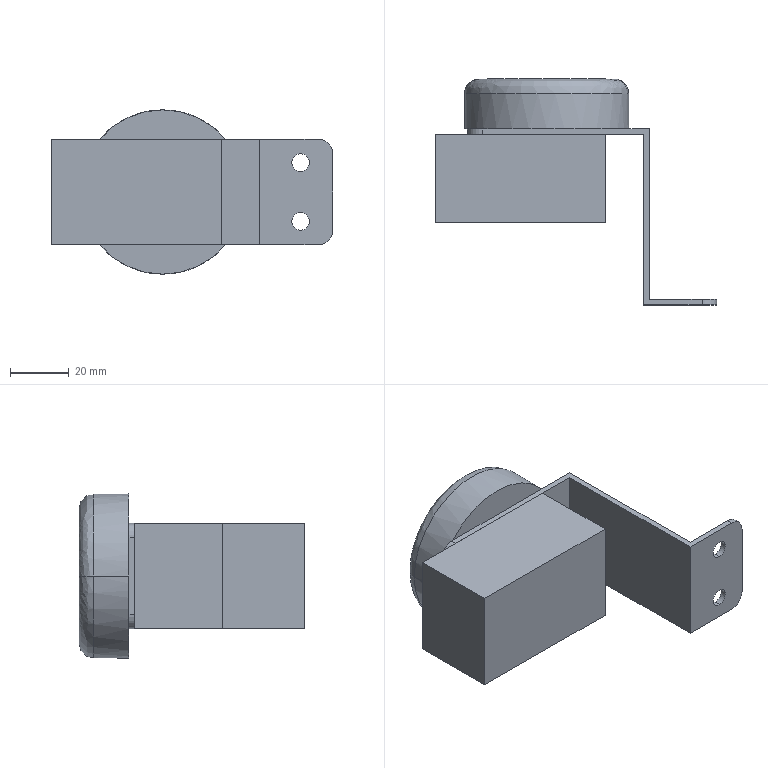Part | STEP file | 750039230 | 2 solids | 34 faces | box 96 x 77 x 56 mm | volume 113749 mm3 | plane 22 | cylinder 10 | spline 2 | commonest cylinder face diameters 6 x4 10 x4 56 x2
STEP:
#1=CARTESIAN_POINT('',(-56.,77.,0.));
#2=VERTEX_POINT('',#1);
#3=CARTESIAN_POINT('',(-10.,77.,0.));
#4=VERTEX_POINT('',#3);
#5=CARTESIAN_POINT('',(-56.,77.,0.));
#6=CARTESIAN_POINT('',(-56.,77.,-46.));
#7=CARTESIAN_POINT('',(-10.,77.,-46.));
#8=CARTESIAN_POINT('',(-10.,77.,0.));
#9=(BOUNDED_CURVE()B_SPLINE_CURVE(3,(#5,#6,#7,#8),.UNSPECIFIED.,.F.,.F.)B_SPLINE_CURVE_WITH_KNOTS((4,4),(0.,0.5),.UNSPECIFIED.)CURVE()GEOMETRIC_REPRESENTATION_ITEM()RATIONAL_B_SPLINE_CURVE((1.,0.3333,0.3333,1.))REPRESENTATION_ITEM(''));
#10=EDGE_CURVE('',#2,#4,#9,.T.);
#11=ORIENTED_EDGE('',*,*,#10,.T.);
#12=CARTESIAN_POINT('',(-5.,72.,0.));
#13=VERTEX_POINT('',#12);
#14=CARTESIAN_POINT('',(-10.,72.,0.));
#15=DIRECTION('',(0.,0.,-1.));
#16=DIRECTION('',(1.,0.,0.));
#17=AXIS2_PLACEMENT_3D('',#14,#15,#16);
#18=CIRCLE('',#17,5.);
#19=EDGE_CURVE('',#4,#13,#18,.T.);
#20=ORIENTED_EDGE('',*,*,#19,.T.);
#21=CARTESIAN_POINT('',(-61.,72.,0.));
#22=VERTEX_POINT('',#21);
#23=CARTESIAN_POINT('',(-33.,72.,0.));
#24=DIRECTION('',(0.,-1.,0.));
#25=DIRECTION('',(1.,0.,0.));
#26=AXIS2_PLACEMENT_3D('',#23,#24,#25);
#27=CIRCLE('',#26,28.);
#28=EDGE_CURVE('',#22,#13,#27,.T.);
#29=ORIENTED_EDGE('',*,*,#28,.F.);
#30=CARTESIAN_POINT('',(-56.,72.,0.));
#31=DIRECTION('',(0.,0.,1.));
#32=DIRECTION('',(-1.,0.,0.));
#33=AXIS2_PLACEMENT_3D('',#30,#31,#32);
#34=CIRCLE('',#33,5.);
#35=EDGE_CURVE('',#2,#22,#34,.T.);
#36=ORIENTED_EDGE('',*,*,#35,.F.);
#37=EDGE_LOOP('',(#11,#20,#29,#36));
#38=FACE_OUTER_BOUND('',#37,.T.);
#39=CARTESIAN_POINT('',(-10.,77.,0.));
#40=CARTESIAN_POINT('',(-10.,77.,-46.));
#41=CARTESIAN_POINT('',(-56.,77.,-46.));
#42=CARTESIAN_POINT('',(-56.,77.,0.));
#43=CARTESIAN_POINT('',(-7.071,77.,0.));
#44=CARTESIAN_POINT('',(-7.071,77.,-51.858));
#45=CARTESIAN_POINT('',(-58.929,77.,-51.858));
#46=CARTESIAN_POINT('',(-58.929,77.,0.));
#47=CARTESIAN_POINT('',(-5.,74.929,0.));
#48=CARTESIAN_POINT('',(-5.,74.929,-56.));
#49=CARTESIAN_POINT('',(-61.,74.929,-56.));
#50=CARTESIAN_POINT('',(-61.,74.929,0.));
#51=CARTESIAN_POINT('',(-5.,72.,0.));
#52=CARTESIAN_POINT('',(-5.,72.,-56.));
#53=CARTESIAN_POINT('',(-61.,72.,-56.));
#54=CARTESIAN_POINT('',(-61.,72.,0.));
#55=(BOUNDED_SURFACE()B_SPLINE_SURFACE(3,3,((#39,#40,#41,#42),(#43,#44,#45,#46),(#47,#48,#49,#50),(#51,#52,#53,#54)),.UNSPECIFIED.,.F.,.F.,.F.)B_SPLINE_SURFACE_WITH_KNOTS((4,4),(4,4),(0.,1.),(0.,1.),.UNSPECIFIED.)GEOMETRIC_REPRESENTATION_ITEM()RATIONAL_B_SPLINE_SURFACE(((1.,0.3333,0.3333,1.),(0.8047,0.2682,0.2682,0.8047),(0.8047,0.2682,0.2682,0.8047),(1.,0.3333,0.3333,1.)))REPRESENTATION_ITEM('')SURFACE());
#56=ADVANCED_FACE('',(#38),#55,.T.);
#57=CARTESIAN_POINT('',(-33.,72.,0.));
#58=DIRECTION('',(0.,-1.,0.));
#59=DIRECTION('',(1.,0.,0.));
#60=AXIS2_PLACEMENT_3D('',#57,#58,#59);
#61=CIRCLE('',#60,28.);
#62=EDGE_CURVE('',#13,#22,#61,.T.);
#63=ORIENTED_EDGE('',*,*,#62,.T.);
#64=CARTESIAN_POINT('',(-61.,60.,0.));
#65=VERTEX_POINT('',#64);
#66=CARTESIAN_POINT('',(-61.,77.,0.));
#67=DIRECTION('',(0.,-1.,0.));
#68=VECTOR('',#67,1000.);
#69=LINE('',#66,#68);
#70=EDGE_CURVE('',#22,#65,#69,.T.);
#71=ORIENTED_EDGE('',*,*,#70,.T.);
#72=CARTESIAN_POINT('',(-60.,60.,7.416));
#73=VERTEX_POINT('',#72);
#74=CARTESIAN_POINT('',(-33.,60.,0.));
#75=DIRECTION('',(0.,1.,0.));
#76=DIRECTION('',(1.,0.,0.));
#77=AXIS2_PLACEMENT_3D('',#74,#75,#76);
#78=CIRCLE('',#77,28.);
#79=EDGE_CURVE('',#65,#73,#78,.T.);
#80=ORIENTED_EDGE('',*,*,#79,.T.);
#81=CARTESIAN_POINT('',(-54.448,60.,18.));
#82=VERTEX_POINT('',#81);
#83=CARTESIAN_POINT('',(-33.,60.,0.));
#84=DIRECTION('',(0.,1.,0.));
#85=DIRECTION('',(1.,0.,0.));
#86=AXIS2_PLACEMENT_3D('',#83,#84,#85);
#87=CIRCLE('',#86,28.);
#88=EDGE_CURVE('',#73,#82,#87,.T.);
#89=ORIENTED_EDGE('',*,*,#88,.T.);
#90=CARTESIAN_POINT('',(-11.552,60.,18.));
#91=VERTEX_POINT('',#90);
#92=CARTESIAN_POINT('',(-33.,60.,0.));
#93=DIRECTION('',(0.,1.,0.));
#94=DIRECTION('',(1.,0.,0.));
#95=AXIS2_PLACEMENT_3D('',#92,#93,#94);
#96=CIRCLE('',#95,28.);
#97=EDGE_CURVE('',#82,#91,#96,.T.);
#98=ORIENTED_EDGE('',*,*,#97,.T.);
#99=CARTESIAN_POINT('',(-5.,60.,0.));
#100=VERTEX_POINT('',#99);
#101=CARTESIAN_POINT('',(-33.,60.,0.));
#102=DIRECTION('',(0.,1.,0.));
#103=DIRECTION('',(1.,0.,0.));
#104=AXIS2_PLACEMENT_3D('',#101,#102,#103);
#105=CIRCLE('',#104,28.);
#106=EDGE_CURVE('',#91,#100,#105,.T.);
#107=ORIENTED_EDGE('',*,*,#106,.T.);
#108=CARTESIAN_POINT('',(-5.,77.,0.));
#109=DIRECTION('',(0.,-1.,0.));
#110=VECTOR('',#109,1000.);
#111=LINE('',#108,#110);
#112=EDGE_CURVE('',#13,#100,#111,.T.);
#113=ORIENTED_EDGE('',*,*,#112,.F.);
#114=EDGE_LOOP('',(#63,#71,#80,#89,#98,#107,#113));
#115=FACE_OUTER_BOUND('',#114,.T.);
#116=CARTESIAN_POINT('',(-33.,77.,0.));
#117=DIRECTION('',(0.,-1.,0.));
#118=DIRECTION('',(1.,0.,0.));
#119=AXIS2_PLACEMENT_3D('',#116,#117,#118);
#120=CYLINDRICAL_SURFACE('',#119,28.);
#121=ADVANCED_FACE('',(#115),#120,.T.);
#122=CARTESIAN_POINT('',(14.,2.,-13.));
#123=VERTEX_POINT('',#122);
#124=CARTESIAN_POINT('',(14.,2.,-7.));
#125=VERTEX_POINT('',#124);
#126=CARTESIAN_POINT('',(14.,2.,-10.));
#127=DIRECTION('',(0.,1.,0.));
#128=DIRECTION('',(0.,0.,-1.));
#129=AXIS2_PLACEMENT_3D('',#126,#127,#128);
#130=CIRCLE('',#129,3.);
#131=EDGE_CURVE('',#123,#125,#130,.T.);
#132=ORIENTED_EDGE('',*,*,#131,.T.);
#133=CARTESIAN_POINT('',(14.,0.,-7.));
#134=VERTEX_POINT('',#133);
#135=CARTESIAN_POINT('',(14.,2.,-7.));
#136=DIRECTION('',(0.,-1.,0.));
#137=VECTOR('',#136,1000.);
#138=LINE('',#135,#137);
#139=EDGE_CURVE('',#125,#134,#138,.T.);
#140=ORIENTED_EDGE('',*,*,#139,.T.);
#141=CARTESIAN_POINT('',(14.,0.,-13.));
#142=VERTEX_POINT('',#141);
#143=CARTESIAN_POINT('',(14.,0.,-10.));
#144=DIRECTION('',(0.,-1.,0.));
#145=DIRECTION('',(0.,0.,-1.));
#146=AXIS2_PLACEMENT_3D('',#143,#144,#145);
#147=CIRCLE('',#146,3.);
#148=EDGE_CURVE('',#134,#142,#147,.T.);
#149=ORIENTED_EDGE('',*,*,#148,.T.);
#150=CARTESIAN_POINT('',(14.,2.,-13.));
#151=DIRECTION('',(0.,-1.,0.));
#152=VECTOR('',#151,1000.);
#153=LINE('',#150,#152);
#154=EDGE_CURVE('',#123,#142,#153,.T.);
#155=ORIENTED_EDGE('',*,*,#154,.F.);
#156=EDGE_LOOP('',(#132,#140,#149,#155));
#157=FACE_OUTER_BOUND('',#156,.T.);
#158=CARTESIAN_POINT('',(14.,2.,-10.));
#159=DIRECTION('',(0.,-1.,0.));
#160=DIRECTION('',(0.,0.,-1.));
#161=AXIS2_PLACEMENT_3D('',#158,#159,#160);
#162=CYLINDRICAL_SURFACE('',#161,3.);
#163=ADVANCED_FACE('',(#157),#162,.F.);
#164=CARTESIAN_POINT('',(14.,2.,7.));
#165=VERTEX_POINT('',#164);
#166=CARTESIAN_POINT('',(14.,2.,13.));
#167=VERTEX_POINT('',#166);
#168=CARTESIAN_POINT('',(14.,2.,10.));
#169=DIRECTION('',(0.,1.,0.));
#170=DIRECTION('',(0.,0.,-1.));
#171=AXIS2_PLACEMENT_3D('',#168,#169,#170);
#172=CIRCLE('',#171,3.);
#173=EDGE_CURVE('',#165,#167,#172,.T.);
#174=ORIENTED_EDGE('',*,*,#173,.T.);
#175=CARTESIAN_POINT('',(14.,0.,13.));
#176=VERTEX_POINT('',#175);
#177=CARTESIAN_POINT('',(14.,2.,13.));
#178=DIRECTION('',(0.,-1.,0.));
#179=VECTOR('',#178,1000.);
#180=LINE('',#177,#179);
#181=EDGE_CURVE('',#167,#176,#180,.T.);
#182=ORIENTED_EDGE('',*,*,#181,.T.);
#183=CARTESIAN_POINT('',(14.,0.,7.));
#184=VERTEX_POINT('',#183);
#185=CARTESIAN_POINT('',(14.,0.,10.));
#186=DIRECTION('',(0.,-1.,0.));
#187=DIRECTION('',(0.,0.,-1.));
#188=AXIS2_PLACEMENT_3D('',#185,#186,#187);
#189=CIRCLE('',#188,3.);
#190=EDGE_CURVE('',#176,#184,#189,.T.);
#191=ORIENTED_EDGE('',*,*,#190,.T.);
#192=CARTESIAN_POINT('',(14.,2.,7.));
#193=DIRECTION('',(0.,-1.,0.));
#194=VECTOR('',#193,1000.);
#195=LINE('',#192,#194);
#196=EDGE_CURVE('',#165,#184,#195,.T.);
#197=ORIENTED_EDGE('',*,*,#196,.F.);
#198=EDGE_LOOP('',(#174,#182,#191,#197));
#199=FACE_OUTER_BOUND('',#198,.T.);
#200=CARTESIAN_POINT('',(14.,2.,10.));
#201=DIRECTION('',(0.,-1.,0.));
#202=DIRECTION('',(0.,0.,-1.));
#203=AXIS2_PLACEMENT_3D('',#200,#201,#202);
#204=CYLINDRICAL_SURFACE('',#203,3.);
#205=ADVANCED_FACE('',(#199),#204,.F.);
#206=CARTESIAN_POINT('',(-60.,58.,13.));
#207=VERTEX_POINT('',#206);
#208=CARTESIAN_POINT('',(-55.,58.,18.));
#209=VERTEX_POINT('',#208);
#210=CARTESIAN_POINT('',(-55.,58.,13.));
#211=DIRECTION('',(0.,1.,0.));
#212=DIRECTION('',(-1.,0.,0.));
#213=AXIS2_PLACEMENT_3D('',#210,#211,#212);
#214=CIRCLE('',#213,5.);
#215=EDGE_CURVE('',#207,#209,#214,.T.);
#216=ORIENTED_EDGE('',*,*,#215,.F.);
#217=CARTESIAN_POINT('',(-60.,58.,-13.));
#218=VERTEX_POINT('',#217);
#219=CARTESIAN_POINT('',(-60.,58.,18.));
#220=DIRECTION('',(0.,0.,1.));
#221=VECTOR('',#220,1000.);
#222=LINE('',#219,#221);
#223=EDGE_CURVE('',#218,#207,#222,.T.);
#224=ORIENTED_EDGE('',*,*,#223,.F.);
#225=CARTESIAN_POINT('',(-55.,58.,-18.));
#226=VERTEX_POINT('',#225);
#227=CARTESIAN_POINT('',(-55.,58.,-13.));
#228=DIRECTION('',(0.,1.,0.));
#229=DIRECTION('',(1.,0.,0.));
#230=AXIS2_PLACEMENT_3D('',#227,#228,#229);
#231=CIRCLE('',#230,5.);
#232=EDGE_CURVE('',#226,#218,#231,.T.);
#233=ORIENTED_EDGE('',*,*,#232,.F.);
#234=CARTESIAN_POINT('',(0.,58.,-18.));
#235=VERTEX_POINT('',#234);
#236=CARTESIAN_POINT('',(-60.,58.,-18.));
#237=DIRECTION('',(-1.,0.,0.));
#238=VECTOR('',#237,1000.);
#239=LINE('',#236,#238);
#240=EDGE_CURVE('',#235,#226,#239,.T.);
#241=ORIENTED_EDGE('',*,*,#240,.F.);
#242=CARTESIAN_POINT('',(0.,58.,18.));
#243=VERTEX_POINT('',#242);
#244=CARTESIAN_POINT('',(0.,58.,18.));
#245=DIRECTION('',(0.,0.,-1.));
#246=VECTOR('',#245,1000.);
#247=LINE('',#244,#246);
#248=EDGE_CURVE('',#243,#235,#247,.T.);
#249=ORIENTED_EDGE('',*,*,#248,.F.);
#250=CARTESIAN_POINT('',(-60.,58.,18.));
#251=DIRECTION('',(1.,0.,0.));
#252=VECTOR('',#251,1000.);
#253=LINE('',#250,#252);
#254=EDGE_CURVE('',#209,#243,#253,.T.);
#255=ORIENTED_EDGE('',*,*,#254,.F.);
#256=EDGE_LOOP('',(#216,#224,#233,#241,#249,#255));
#257=FACE_OUTER_BOUND('',#256,.T.);
#258=CARTESIAN_POINT('',(-60.,58.,18.));
#259=DIRECTION('',(0.,1.,0.));
#260=DIRECTION('',(-1.,0.,0.));
#261=AXIS2_PLACEMENT_3D('',#258,#259,#260);
#262=PLANE('',#261);
#263=ADVANCED_FACE('',(#257),#262,.F.);
#264=CARTESIAN_POINT('',(2.,60.,18.));
#265=VERTEX_POINT('',#264);
#266=CARTESIAN_POINT('',(0.,60.,18.));
#267=DIRECTION('',(-1.,0.,0.));
#268=VECTOR('',#267,1000.);
#269=LINE('',#266,#268);
#270=EDGE_CURVE('',#265,#91,#269,.T.);
#271=ORIENTED_EDGE('',*,*,#270,.T.);
#272=CARTESIAN_POINT('',(0.,60.,18.));
#273=DIRECTION('',(-1.,0.,0.));
#274=VECTOR('',#273,1000.);
#275=LINE('',#272,#274);
#276=EDGE_CURVE('',#91,#82,#275,.T.);
#277=ORIENTED_EDGE('',*,*,#276,.T.);
#278=CARTESIAN_POINT('',(-55.,60.,18.));
#279=VERTEX_POINT('',#278);
#280=CARTESIAN_POINT('',(2.,60.,18.));
#281=DIRECTION('',(-1.,0.,0.));
#282=VECTOR('',#281,1000.);
#283=LINE('',#280,#282);
#284=EDGE_CURVE('',#82,#279,#283,.T.);
#285=ORIENTED_EDGE('',*,*,#284,.T.);
#286=CARTESIAN_POINT('',(-55.,0.,18.));
#287=DIRECTION('',(0.,-1.,0.));
#288=VECTOR('',#287,1000.);
#289=LINE('',#286,#288);
#290=EDGE_CURVE('',#279,#209,#289,.T.);
#291=ORIENTED_EDGE('',*,*,#290,.T.);
#292=ORIENTED_EDGE('',*,*,#254,.T.);
#293=CARTESIAN_POINT('',(0.,0.,18.));
#294=VERTEX_POINT('',#293);
#295=CARTESIAN_POINT('',(0.,0.,18.));
#296=DIRECTION('',(0.,-1.,0.));
#297=VECTOR('',#296,1000.);
#298=LINE('',#295,#297);
#299=EDGE_CURVE('',#243,#294,#298,.T.);
#300=ORIENTED_EDGE('',*,*,#299,.T.);
#301=CARTESIAN_POINT('',(20.,0.,18.));
#302=VERTEX_POINT('',#301);
#303=CARTESIAN_POINT('',(0.,0.,18.));
#304=DIRECTION('',(1.,0.,0.));
#305=VECTOR('',#304,1000.);
#306=LINE('',#303,#305);
#307=EDGE_CURVE('',#294,#302,#306,.T.);
#308=ORIENTED_EDGE('',*,*,#307,.T.);
#309=CARTESIAN_POINT('',(20.,2.,18.));
#310=VERTEX_POINT('',#309);
#311=CARTESIAN_POINT('',(20.,0.,18.));
#312=DIRECTION('',(0.,1.,0.));
#313=VECTOR('',#312,1000.);
#314=LINE('',#311,#313);
#315=EDGE_CURVE('',#302,#310,#314,.T.);
#316=ORIENTED_EDGE('',*,*,#315,.T.);
#317=CARTESIAN_POINT('',(2.,2.,18.));
#318=VERTEX_POINT('',#317);
#319=CARTESIAN_POINT('',(0.,2.,18.));
#320=DIRECTION('',(-1.,0.,0.));
#321=VECTOR('',#320,1000.);
#322=LINE('',#319,#321);
#323=EDGE_CURVE('',#310,#318,#322,.T.);
#324=ORIENTED_EDGE('',*,*,#323,.T.);
#325=CARTESIAN_POINT('',(2.,0.,18.));
#326=DIRECTION('',(0.,1.,0.));
#327=VECTOR('',#326,1000.);
#328=LINE('',#325,#327);
#329=EDGE_CURVE('',#318,#265,#328,.T.);
#330=ORIENTED_EDGE('',*,*,#329,.T.);
#331=EDGE_LOOP('',(#271,#277,#285,#291,#292,#300,#308,#316,#324,#330));
#332=FACE_OUTER_BOUND('',#331,.T.);
#333=CARTESIAN_POINT('',(0.,0.,18.));
#334=DIRECTION('',(0.,0.,1.));
#335=DIRECTION('',(1.,0.,0.));
#336=AXIS2_PLACEMENT_3D('',#333,#334,#335);
#337=PLANE('',#336);
#338=ADVANCED_FACE('',(#332),#337,.T.);
#339=ORIENTED_EDGE('',*,*,#215,.T.);
#340=ORIENTED_EDGE('',*,*,#290,.F.);
#341=CARTESIAN_POINT('',(-60.,60.,13.));
#342=VERTEX_POINT('',#341);
#343=CARTESIAN_POINT('',(-55.,60.,13.));
#344=DIRECTION('',(0.,-1.,0.));
#345=DIRECTION('',(-1.,0.,0.));
#346=AXIS2_PLACEMENT_3D('',#343,#344,#345);
#347=CIRCLE('',#346,5.);
#348=EDGE_CURVE('',#279,#342,#347,.T.);
#349=ORIENTED_EDGE('',*,*,#348,.T.);
#350=CARTESIAN_POINT('',(-60.,0.,13.));
#351=DIRECTION('',(0.,-1.,0.));
#352=VECTOR('',#351,1000.);
#353=LINE('',#350,#352);
#354=EDGE_CURVE('',#342,#207,#353,.T.);
#355=ORIENTED_EDGE('',*,*,#354,.T.);
#356=EDGE_LOOP('',(#339,#340,#349,#355));
#357=FACE_OUTER_BOUND('',#356,.T.);
#358=CARTESIAN_POINT('',(-55.,0.,13.));
#359=DIRECTION('',(0.,1.,0.));
#360=DIRECTION('',(-1.,0.,0.));
#361=AXIS2_PLACEMENT_3D('',#358,#359,#360);
#362=CYLINDRICAL_SURFACE('',#361,5.);
#363=ADVANCED_FACE('',(#357),#362,.T.);
#364=ORIENTED_EDGE('',*,*,#354,.F.);
#365=CARTESIAN_POINT('',(-60.,60.,18.));
#366=DIRECTION('',(0.,0.,1.));
#367=VECTOR('',#366,1000.);
#368=LINE('',#365,#367);
#369=EDGE_CURVE('',#73,#342,#368,.T.);
#370=ORIENTED_EDGE('',*,*,#369,.F.);
#371=CARTESIAN_POINT('',(-60.,60.,-7.416));
#372=VERTEX_POINT('',#371);
#373=CARTESIAN_POINT('',(-60.,60.,18.));
#374=DIRECTION('',(0.,0.,1.));
#375=VECTOR('',#374,1000.);
#376=LINE('',#373,#375);
#377=EDGE_CURVE('',#372,#73,#376,.T.);
#378=ORIENTED_EDGE('',*,*,#377,.F.);
#379=CARTESIAN_POINT('',(-60.,60.,-13.));
#380=VERTEX_POINT('',#379);
#381=CARTESIAN_POINT('',(-60.,60.,18.));
#382=DIRECTION('',(0.,0.,1.));
#383=VECTOR('',#382,1000.);
#384=LINE('',#381,#383);
#385=EDGE_CURVE('',#380,#372,#384,.T.);
#386=ORIENTED_EDGE('',*,*,#385,.F.);
#387=CARTESIAN_POINT('',(-60.,60.,-13.));
#388=DIRECTION('',(0.,1.,0.));
#389=VECTOR('',#388,1000.);
#390=LINE('',#387,#389);
#391=EDGE_CURVE('',#218,#380,#390,.T.);
#392=ORIENTED_EDGE('',*,*,#391,.F.);
#393=ORIENTED_EDGE('',*,*,#223,.T.);
#394=EDGE_LOOP('',(#364,#370,#378,#386,#392,#393));
#395=FACE_OUTER_BOUND('',#394,.T.);
#396=CARTESIAN_POINT('',(-60.,60.,18.));
#397=DIRECTION('',(1.,0.,0.));
#398=DIRECTION('',(0.,1.,0.));
#399=AXIS2_PLACEMENT_3D('',#396,#397,#398);
#400=PLANE('',#399);
#401=ADVANCED_FACE('',(#395),#400,.F.);
#402=ORIENTED_EDGE('',*,*,#232,.T.);
#403=ORIENTED_EDGE('',*,*,#391,.T.);
#404=CARTESIAN_POINT('',(-55.,60.,-18.));
#405=VERTEX_POINT('',#404);
#406=CARTESIAN_POINT('',(-55.,60.,-13.));
#407=DIRECTION('',(0.,-1.,0.));
#408=DIRECTION('',(1.,0.,0.));
#409=AXIS2_PLACEMENT_3D('',#406,#407,#408);
#410=CIRCLE('',#409,5.);
#411=EDGE_CURVE('',#380,#405,#410,.T.);
#412=ORIENTED_EDGE('',*,*,#411,.T.);
#413=CARTESIAN_POINT('',(-55.,60.,-18.));
#414=DIRECTION('',(0.,-1.,0.));
#415=VECTOR('',#414,1000.);
#416=LINE('',#413,#415);
#417=EDGE_CURVE('',#405,#226,#416,.T.);
#418=ORIENTED_EDGE('',*,*,#417,.T.);
#419=EDGE_LOOP('',(#402,#403,#412,#418));
#420=FACE_OUTER_BOUND('',#419,.T.);
#421=CARTESIAN_POINT('',(-55.,60.,-13.));
#422=DIRECTION('',(0.,-1.,0.));
#423=DIRECTION('',(1.,0.,0.));
#424=AXIS2_PLACEMENT_3D('',#421,#422,#423);
#425=CYLINDRICAL_SURFACE('',#424,5.);
#426=ADVANCED_FACE('',(#420),#425,.T.);
#427=ORIENTED_EDGE('',*,*,#417,.F.);
#428=CARTESIAN_POINT('',(-54.448,60.,-18.));
#429=VERTEX_POINT('',#428);
#430=CARTESIAN_POINT('',(0.,60.,-18.));
#431=DIRECTION('',(-1.,0.,0.));
#432=VECTOR('',#431,1000.);
#433=LINE('',#430,#432);
#434=EDGE_CURVE('',#429,#405,#433,.T.);
#435=ORIENTED_EDGE('',*,*,#434,.F.);
#436=CARTESIAN_POINT('',(-11.552,60.,-18.));
#437=VERTEX_POINT('',#436);
#438=CARTESIAN_POINT('',(0.,60.,-18.));
#439=DIRECTION('',(-1.,0.,0.));
#440=VECTOR('',#439,1000.);
#441=LINE('',#438,#440);
#442=EDGE_CURVE('',#437,#429,#441,.T.);
#443=ORIENTED_EDGE('',*,*,#442,.F.);
#444=CARTESIAN_POINT('',(2.,60.,-18.));
#445=VERTEX_POINT('',#444);
#446=CARTESIAN_POINT('',(0.,60.,-18.));
#447=DIRECTION('',(-1.,0.,0.));
#448=VECTOR('',#447,1000.);
#449=LINE('',#446,#448);
#450=EDGE_CURVE('',#445,#437,#449,.T.);
#451=ORIENTED_EDGE('',*,*,#450,.F.);
#452=CARTESIAN_POINT('',(2.,2.,-18.));
#453=VERTEX_POINT('',#452);
#454=CARTESIAN_POINT('',(2.,0.,-18.));
#455=DIRECTION('',(0.,1.,0.));
#456=VECTOR('',#455,1000.);
#457=LINE('',#454,#456);
#458=EDGE_CURVE('',#453,#445,#457,.T.);
#459=ORIENTED_EDGE('',*,*,#458,.F.);
#460=CARTESIAN_POINT('',(20.,2.,-18.));
#461=VERTEX_POINT('',#460);
#462=CARTESIAN_POINT('',(0.,2.,-18.));
#463=DIRECTION('',(-1.,0.,0.));
#464=VECTOR('',#463,1000.);
#465=LINE('',#462,#464);
#466=EDGE_CURVE('',#461,#453,#465,.T.);
#467=ORIENTED_EDGE('',*,*,#466,.F.);
#468=CARTESIAN_POINT('',(20.,0.,-18.));
#469=VERTEX_POINT('',#468);
#470=CARTESIAN_POINT('',(20.,0.,-18.));
#471=DIRECTION('',(0.,1.,0.));
#472=VECTOR('',#471,1000.);
#473=LINE('',#470,#472);
#474=EDGE_CURVE('',#469,#461,#473,.T.);
#475=ORIENTED_EDGE('',*,*,#474,.F.);
#476=CARTESIAN_POINT('',(0.,0.,-18.));
#477=VERTEX_POINT('',#476);
#478=CARTESIAN_POINT('',(0.,0.,-18.));
#479=DIRECTION('',(1.,0.,0.));
#480=VECTOR('',#479,1000.);
#481=LINE('',#478,#480);
#482=EDGE_CURVE('',#477,#469,#481,.T.);
#483=ORIENTED_EDGE('',*,*,#482,.F.);
#484=CARTESIAN_POINT('',(0.,0.,-18.));
#485=DIRECTION('',(0.,-1.,0.));
#486=VECTOR('',#485,1000.);
#487=LINE('',#484,#486);
#488=EDGE_CURVE('',#235,#477,#487,.T.);
#489=ORIENTED_EDGE('',*,*,#488,.F.);
#490=ORIENTED_EDGE('',*,*,#240,.T.);
#491=EDGE_LOOP('',(#427,#435,#443,#451,#459,#467,#475,#483,#489,#490));
#492=FACE_OUTER_BOUND('',#491,.T.);
#493=CARTESIAN_POINT('',(0.,0.,-18.));
#494=DIRECTION('',(0.,0.,1.));
#495=DIRECTION('',(1.,0.,0.));
#496=AXIS2_PLACEMENT_3D('',#493,#494,#495);
#497=PLANE('',#496);
#498=ADVANCED_FACE('',(#492),#497,.F.);
#499=CARTESIAN_POINT('',(0.,0.,18.));
#500=DIRECTION('',(0.,0.,-1.));
#501=VECTOR('',#500,1000.);
#502=LINE('',#499,#501);
#503=EDGE_CURVE('',#294,#477,#502,.T.);
#504=ORIENTED_EDGE('',*,*,#503,.F.);
#505=ORIENTED_EDGE('',*,*,#299,.F.);
#506=ORIENTED_EDGE('',*,*,#248,.T.);
#507=ORIENTED_EDGE('',*,*,#488,.T.);
#508=EDGE_LOOP('',(#504,#505,#506,#507));
#509=FACE_OUTER_BOUND('',#508,.T.);
#510=CARTESIAN_POINT('',(0.,58.,18.));
#511=DIRECTION('',(1.,0.,0.));
#512=DIRECTION('',(0.,1.,0.));
#513=AXIS2_PLACEMENT_3D('',#510,#511,#512);
#514=PLANE('',#513);
#515=ADVANCED_FACE('',(#509),#514,.F.);
#516=ORIENTED_EDGE('',*,*,#97,.F.);
#517=ORIENTED_EDGE('',*,*,#276,.F.);
#518=EDGE_LOOP('',(#516,#517));
#519=FACE_OUTER_BOUND('',#518,.T.);
#520=CARTESIAN_POINT('',(-33.,60.,0.));
#521=DIRECTION('',(0.,1.,0.));
#522=DIRECTION('',(-1.,0.,0.));
#523=AXIS2_PLACEMENT_3D('',#520,#521,#522);
#524=PLANE('',#523);
#525=ADVANCED_FACE('',(#519),#524,.F.);
#526=ORIENTED_EDGE('',*,*,#270,.F.);
#527=CARTESIAN_POINT('',(2.,60.,18.));
#528=DIRECTION('',(0.,0.,1.));
#529=VECTOR('',#528,1000.);
#530=LINE('',#527,#529);
#531=EDGE_CURVE('',#445,#265,#530,.T.);
#532=ORIENTED_EDGE('',*,*,#531,.F.);
#533=ORIENTED_EDGE('',*,*,#450,.T.);
#534=CARTESIAN_POINT('',(-33.,60.,0.));
#535=DIRECTION('',(0.,1.,0.));
#536=DIRECTION('',(1.,0.,0.));
#537=AXIS2_PLACEMENT_3D('',#534,#535,#536);
#538=CIRCLE('',#537,28.);
#539=EDGE_CURVE('',#100,#437,#538,.T.);
#540=ORIENTED_EDGE('',*,*,#539,.F.);
#541=ORIENTED_EDGE('',*,*,#106,.F.);
#542=EDGE_LOOP('',(#526,#532,#533,#540,#541));
#543=FACE_OUTER_BOUND('',#542,.T.);
#544=CARTESIAN_POINT('',(2.,60.,18.));
#545=DIRECTION('',(0.,-1.,0.));
#546=DIRECTION('',(1.,0.,0.));
#547=AXIS2_PLACEMENT_3D('',#544,#545,#546);
#548=PLANE('',#547);
#549=ADVANCED_FACE('',(#543),#548,.F.);
#550=ORIENTED_EDGE('',*,*,#531,.T.);
#551=ORIENTED_EDGE('',*,*,#329,.F.);
#552=CARTESIAN_POINT('',(2.,2.,18.));
#553=DIRECTION('',(0.,0.,1.));
#554=VECTOR('',#553,1000.);
#555=LINE('',#552,#554);
#556=EDGE_CURVE('',#453,#318,#555,.T.);
#557=ORIENTED_EDGE('',*,*,#556,.F.);
#558=ORIENTED_EDGE('',*,*,#458,.T.);
#559=EDGE_LOOP('',(#550,#551,#557,#558));
#560=FACE_OUTER_BOUND('',#559,.T.);
#561=CARTESIAN_POINT('',(2.,2.,18.));
#562=DIRECTION('',(-1.,0.,0.));
#563=DIRECTION('',(0.,-1.,0.));
#564=AXIS2_PLACEMENT_3D('',#561,#562,#563);
#565=PLANE('',#564);
#566=ADVANCED_FACE('',(#560),#565,.F.);
#567=ORIENTED_EDGE('',*,*,#131,.F.);
#568=CARTESIAN_POINT('',(14.,2.,-10.));
#569=DIRECTION('',(0.,1.,0.));
#570=DIRECTION('',(0.,0.,-1.));
#571=AXIS2_PLACEMENT_3D('',#568,#569,#570);
#572=CIRCLE('',#571,3.);
#573=EDGE_CURVE('',#125,#123,#572,.T.);
#574=ORIENTED_EDGE('',*,*,#573,.F.);
#575=EDGE_LOOP('',(#567,#574));
#576=FACE_BOUND('',#575,.T.);
#577=CARTESIAN_POINT('',(25.,2.,13.));
#578=VERTEX_POINT('',#577);
#579=CARTESIAN_POINT('',(20.,2.,13.));
#580=DIRECTION('',(0.,-1.,0.));
#581=DIRECTION('',(1.,0.,0.));
#582=AXIS2_PLACEMENT_3D('',#579,#580,#581);
#583=CIRCLE('',#582,5.);
#584=EDGE_CURVE('',#578,#310,#583,.T.);
#585=ORIENTED_EDGE('',*,*,#584,.F.);
#586=CARTESIAN_POINT('',(25.,2.,-13.));
#587=VERTEX_POINT('',#586);
#588=CARTESIAN_POINT('',(25.,2.,18.));
#589=DIRECTION('',(0.,0.,1.));
#590=VECTOR('',#589,1000.);
#591=LINE('',#588,#590);
#592=EDGE_CURVE('',#587,#578,#591,.T.);
#593=ORIENTED_EDGE('',*,*,#592,.F.);
#594=CARTESIAN_POINT('',(20.,2.,-13.));
#595=DIRECTION('',(0.,-1.,0.));
#596=DIRECTION('',(-1.,0.,0.));
#597=AXIS2_PLACEMENT_3D('',#594,#595,#596);
#598=CIRCLE('',#597,5.);
#599=EDGE_CURVE('',#461,#587,#598,.T.);
#600=ORIENTED_EDGE('',*,*,#599,.F.);
#601=ORIENTED_EDGE('',*,*,#466,.T.);
#602=ORIENTED_EDGE('',*,*,#556,.T.);
#603=ORIENTED_EDGE('',*,*,#323,.F.);
#604=EDGE_LOOP('',(#585,#593,#600,#601,#602,#603));
#605=FACE_OUTER_BOUND('',#604,.T.);
#606=ORIENTED_EDGE('',*,*,#173,.F.);
#607=CARTESIAN_POINT('',(14.,2.,10.));
#608=DIRECTION('',(0.,1.,0.));
#609=DIRECTION('',(0.,0.,-1.));
#610=AXIS2_PLACEMENT_3D('',#607,#608,#609);
#611=CIRCLE('',#610,3.);
#612=EDGE_CURVE('',#167,#165,#611,.T.);
#613=ORIENTED_EDGE('',*,*,#612,.F.);
#614=EDGE_LOOP('',(#606,#613));
#615=FACE_BOUND('',#614,.T.);
#616=CARTESIAN_POINT('',(25.,2.,18.));
#617=DIRECTION('',(0.,-1.,0.));
#618=DIRECTION('',(0.,0.,-1.));
#619=AXIS2_PLACEMENT_3D('',#616,#617,#618);
#620=PLANE('',#619);
#621=ADVANCED_FACE('',(#576,#605,#615),#620,.F.);
#622=ORIENTED_EDGE('',*,*,#584,.T.);
#623=ORIENTED_EDGE('',*,*,#315,.F.);
#624=CARTESIAN_POINT('',(25.,0.,13.));
#625=VERTEX_POINT('',#624);
#626=CARTESIAN_POINT('',(20.,0.,13.));
#627=DIRECTION('',(0.,1.,0.));
#628=DIRECTION('',(1.,0.,0.));
#629=AXIS2_PLACEMENT_3D('',#626,#627,#628);
#630=CIRCLE('',#629,5.);
#631=EDGE_CURVE('',#302,#625,#630,.T.);
#632=ORIENTED_EDGE('',*,*,#631,.T.);
#633=CARTESIAN_POINT('',(25.,0.,13.));
#634=DIRECTION('',(0.,1.,0.));
#635=VECTOR('',#634,1000.);
#636=LINE('',#633,#635);
#637=EDGE_CURVE('',#625,#578,#636,.T.);
#638=ORIENTED_EDGE('',*,*,#637,.T.);
#639=EDGE_LOOP('',(#622,#623,#632,#638));
#640=FACE_OUTER_BOUND('',#639,.T.);
#641=CARTESIAN_POINT('',(20.,0.,13.));
#642=DIRECTION('',(0.,-1.,0.));
#643=DIRECTION('',(1.,0.,0.));
#644=AXIS2_PLACEMENT_3D('',#641,#642,#643);
#645=CYLINDRICAL_SURFACE('',#644,5.);
#646=ADVANCED_FACE('',(#640),#645,.T.);
#647=CARTESIAN_POINT('',(14.,0.,-10.));
#648=DIRECTION('',(0.,-1.,0.));
#649=DIRECTION('',(0.,0.,-1.));
#650=AXIS2_PLACEMENT_3D('',#647,#648,#649);
#651=CIRCLE('',#650,3.);
#652=EDGE_CURVE('',#142,#134,#651,.T.);
#653=ORIENTED_EDGE('',*,*,#652,.F.);
#654=ORIENTED_EDGE('',*,*,#148,.F.);
#655=EDGE_LOOP('',(#653,#654));
#656=FACE_BOUND('',#655,.T.);
#657=CARTESIAN_POINT('',(14.,0.,10.));
#658=DIRECTION('',(0.,-1.,0.));
#659=DIRECTION('',(0.,0.,-1.));
#660=AXIS2_PLACEMENT_3D('',#657,#658,#659);
#661=CIRCLE('',#660,3.);
#662=EDGE_CURVE('',#184,#176,#661,.T.);
#663=ORIENTED_EDGE('',*,*,#662,.F.);
#664=ORIENTED_EDGE('',*,*,#190,.F.);
#665=EDGE_LOOP('',(#663,#664));
#666=FACE_BOUND('',#665,.T.);
#667=ORIENTED_EDGE('',*,*,#631,.F.);
#668=ORIENTED_EDGE('',*,*,#307,.F.);
#669=ORIENTED_EDGE('',*,*,#503,.T.);
#670=ORIENTED_EDGE('',*,*,#482,.T.);
#671=CARTESIAN_POINT('',(25.,0.,-13.));
#672=VERTEX_POINT('',#671);
#673=CARTESIAN_POINT('',(20.,0.,-13.));
#674=DIRECTION('',(0.,1.,0.));
#675=DIRECTION('',(-1.,0.,0.));
#676=AXIS2_PLACEMENT_3D('',#673,#674,#675);
#677=CIRCLE('',#676,5.);
#678=EDGE_CURVE('',#672,#469,#677,.T.);
#679=ORIENTED_EDGE('',*,*,#678,.F.);
#680=CARTESIAN_POINT('',(25.,0.,18.));
#681=DIRECTION('',(0.,0.,-1.));
#682=VECTOR('',#681,1000.);
#683=LINE('',#680,#682);
#684=EDGE_CURVE('',#625,#672,#683,.T.);
#685=ORIENTED_EDGE('',*,*,#684,.F.);
#686=EDGE_LOOP('',(#667,#668,#669,#670,#679,#685));
#687=FACE_OUTER_BOUND('',#686,.T.);
#688=CARTESIAN_POINT('',(0.,0.,18.));
#689=DIRECTION('',(0.,1.,0.));
#690=DIRECTION('',(0.,0.,1.));
#691=AXIS2_PLACEMENT_3D('',#688,#689,#690);
#692=PLANE('',#691);
#693=ADVANCED_FACE('',(#656,#666,#687),#692,.F.);
#694=ORIENTED_EDGE('',*,*,#348,.F.);
#695=ORIENTED_EDGE('',*,*,#284,.F.);
#696=ORIENTED_EDGE('',*,*,#88,.F.);
#697=ORIENTED_EDGE('',*,*,#369,.T.);
#698=EDGE_LOOP('',(#694,#695,#696,#697));
#699=FACE_OUTER_BOUND('',#698,.T.);
#700=CARTESIAN_POINT('',(2.,60.,18.));
#701=DIRECTION('',(0.,-1.,0.));
#702=DIRECTION('',(1.,0.,0.));
#703=AXIS2_PLACEMENT_3D('',#700,#701,#702);
#704=PLANE('',#703);
#705=ADVANCED_FACE('',(#699),#704,.F.);
#706=CARTESIAN_POINT('',(-33.,60.,0.));
#707=DIRECTION('',(0.,1.,0.));
#708=DIRECTION('',(1.,0.,0.));
#709=AXIS2_PLACEMENT_3D('',#706,#707,#708);
#710=CIRCLE('',#709,28.);
#711=EDGE_CURVE('',#372,#65,#710,.T.);
#712=ORIENTED_EDGE('',*,*,#711,.F.);
#713=ORIENTED_EDGE('',*,*,#377,.T.);
#714=ORIENTED_EDGE('',*,*,#79,.F.);
#715=EDGE_LOOP('',(#712,#713,#714));
#716=FACE_OUTER_BOUND('',#715,.T.);
#717=CARTESIAN_POINT('',(-33.,60.,0.));
#718=DIRECTION('',(0.,1.,0.));
#719=DIRECTION('',(-1.,0.,0.));
#720=AXIS2_PLACEMENT_3D('',#717,#718,#719);
#721=PLANE('',#720);
#722=ADVANCED_FACE('',(#716),#721,.F.);
#723=ORIENTED_EDGE('',*,*,#411,.F.);
#724=ORIENTED_EDGE('',*,*,#385,.T.);
#725=CARTESIAN_POINT('',(-33.,60.,0.));
#726=DIRECTION('',(0.,1.,0.));
#727=DIRECTION('',(1.,0.,0.));
#728=AXIS2_PLACEMENT_3D('',#725,#726,#727);
#729=CIRCLE('',#728,28.);
#730=EDGE_CURVE('',#429,#372,#729,.T.);
#731=ORIENTED_EDGE('',*,*,#730,.F.);
#732=ORIENTED_EDGE('',*,*,#434,.T.);
#733=EDGE_LOOP('',(#723,#724,#731,#732));
#734=FACE_OUTER_BOUND('',#733,.T.);
#735=CARTESIAN_POINT('',(2.,60.,18.));
#736=DIRECTION('',(0.,-1.,0.));
#737=DIRECTION('',(1.,0.,0.));
#738=AXIS2_PLACEMENT_3D('',#735,#736,#737);
#739=PLANE('',#738);
#740=ADVANCED_FACE('',(#734),#739,.F.);
#741=ORIENTED_EDGE('',*,*,#442,.T.);
#742=CARTESIAN_POINT('',(-33.,60.,0.));
#743=DIRECTION('',(0.,1.,0.));
#744=DIRECTION('',(1.,0.,0.));
#745=AXIS2_PLACEMENT_3D('',#742,#743,#744);
#746=CIRCLE('',#745,28.);
#747=EDGE_CURVE('',#437,#429,#746,.T.);
#748=ORIENTED_EDGE('',*,*,#747,.F.);
#749=EDGE_LOOP('',(#741,#748));
#750=FACE_OUTER_BOUND('',#749,.T.);
#751=CARTESIAN_POINT('',(-33.,60.,0.));
#752=DIRECTION('',(0.,1.,0.));
#753=DIRECTION('',(-1.,0.,0.));
#754=AXIS2_PLACEMENT_3D('',#751,#752,#753);
#755=PLANE('',#754);
#756=ADVANCED_FACE('',(#750),#755,.F.);
#757=ORIENTED_EDGE('',*,*,#599,.T.);
#758=CARTESIAN_POINT('',(25.,0.,-13.));
#759=DIRECTION('',(0.,-1.,0.));
#760=VECTOR('',#759,1000.);
#761=LINE('',#758,#760);
#762=EDGE_CURVE('',#587,#672,#761,.T.);
#763=ORIENTED_EDGE('',*,*,#762,.T.);
#764=ORIENTED_EDGE('',*,*,#678,.T.);
#765=ORIENTED_EDGE('',*,*,#474,.T.);
#766=EDGE_LOOP('',(#757,#763,#764,#765));
#767=FACE_OUTER_BOUND('',#766,.T.);
#768=CARTESIAN_POINT('',(20.,0.,-13.));
#769=DIRECTION('',(0.,1.,0.));
#770=DIRECTION('',(-1.,0.,0.));
#771=AXIS2_PLACEMENT_3D('',#768,#769,#770);
#772=CYLINDRICAL_SURFACE('',#771,5.);
#773=ADVANCED_FACE('',(#767),#772,.T.);
#774=ORIENTED_EDGE('',*,*,#70,.F.);
#775=ORIENTED_EDGE('',*,*,#28,.T.);
#776=ORIENTED_EDGE('',*,*,#112,.T.);
#777=ORIENTED_EDGE('',*,*,#539,.T.);
#778=ORIENTED_EDGE('',*,*,#747,.T.);
#779=ORIENTED_EDGE('',*,*,#730,.T.);
#780=ORIENTED_EDGE('',*,*,#711,.T.);
#781=EDGE_LOOP('',(#774,#775,#776,#777,#778,#779,#780));
#782=FACE_OUTER_BOUND('',#781,.T.);
#783=CARTESIAN_POINT('',(-33.,77.,0.));
#784=DIRECTION('',(0.,-1.,0.));
#785=DIRECTION('',(1.,0.,0.));
#786=AXIS2_PLACEMENT_3D('',#783,#784,#785);
#787=CYLINDRICAL_SURFACE('',#786,28.);
#788=ADVANCED_FACE('',(#782),#787,.T.);
#789=ORIENTED_EDGE('',*,*,#139,.F.);
#790=ORIENTED_EDGE('',*,*,#573,.T.);
#791=ORIENTED_EDGE('',*,*,#154,.T.);
#792=ORIENTED_EDGE('',*,*,#652,.T.);
#793=EDGE_LOOP('',(#789,#790,#791,#792));
#794=FACE_OUTER_BOUND('',#793,.T.);
#795=CARTESIAN_POINT('',(14.,2.,-10.));
#796=DIRECTION('',(0.,-1.,0.));
#797=DIRECTION('',(0.,0.,-1.));
#798=AXIS2_PLACEMENT_3D('',#795,#796,#797);
#799=CYLINDRICAL_SURFACE('',#798,3.);
#800=ADVANCED_FACE('',(#794),#799,.F.);
#801=ORIENTED_EDGE('',*,*,#637,.F.);
#802=ORIENTED_EDGE('',*,*,#684,.T.);
#803=ORIENTED_EDGE('',*,*,#762,.F.);
#804=ORIENTED_EDGE('',*,*,#592,.T.);
#805=EDGE_LOOP('',(#801,#802,#803,#804));
#806=FACE_OUTER_BOUND('',#805,.T.);
#807=CARTESIAN_POINT('',(25.,0.,18.));
#808=DIRECTION('',(-1.,0.,0.));
#809=DIRECTION('',(0.,-1.,0.));
#810=AXIS2_PLACEMENT_3D('',#807,#808,#809);
#811=PLANE('',#810);
#812=ADVANCED_FACE('',(#806),#811,.F.);
#813=ORIENTED_EDGE('',*,*,#181,.F.);
#814=ORIENTED_EDGE('',*,*,#612,.T.);
#815=ORIENTED_EDGE('',*,*,#196,.T.);
#816=ORIENTED_EDGE('',*,*,#662,.T.);
#817=EDGE_LOOP('',(#813,#814,#815,#816));
#818=FACE_OUTER_BOUND('',#817,.T.);
#819=CARTESIAN_POINT('',(14.,2.,10.));
#820=DIRECTION('',(0.,-1.,0.));
#821=DIRECTION('',(0.,0.,-1.));
#822=AXIS2_PLACEMENT_3D('',#819,#820,#821);
#823=CYLINDRICAL_SURFACE('',#822,3.);
#824=ADVANCED_FACE('',(#818),#823,.F.);
#825=ORIENTED_EDGE('',*,*,#19,.F.);
#826=CARTESIAN_POINT('',(-10.,77.,0.));
#827=CARTESIAN_POINT('',(-10.,77.,46.));
#828=CARTESIAN_POINT('',(-56.,77.,46.));
#829=CARTESIAN_POINT('',(-56.,77.,0.));
#830=(BOUNDED_CURVE()B_SPLINE_CURVE(3,(#826,#827,#828,#829),.UNSPECIFIED.,.F.,.T.)B_SPLINE_CURVE_WITH_KNOTS((4,4),(0.5,1.),.UNSPECIFIED.)CURVE()GEOMETRIC_REPRESENTATION_ITEM()RATIONAL_B_SPLINE_CURVE((1.,0.3333,0.3333,1.))REPRESENTATION_ITEM(''));
#831=EDGE_CURVE('',#4,#2,#830,.T.);
#832=ORIENTED_EDGE('',*,*,#831,.T.);
#833=ORIENTED_EDGE('',*,*,#35,.T.);
#834=ORIENTED_EDGE('',*,*,#62,.F.);
#835=EDGE_LOOP('',(#825,#832,#833,#834));
#836=FACE_OUTER_BOUND('',#835,.T.);
#837=CARTESIAN_POINT('',(-56.,77.,0.));
#838=CARTESIAN_POINT('',(-56.,77.,46.));
#839=CARTESIAN_POINT('',(-10.,77.,46.));
#840=CARTESIAN_POINT('',(-10.,77.,0.));
#841=CARTESIAN_POINT('',(-58.929,77.,0.));
#842=CARTESIAN_POINT('',(-58.929,77.,51.858));
#843=CARTESIAN_POINT('',(-7.071,77.,51.858));
#844=CARTESIAN_POINT('',(-7.071,77.,0.));
#845=CARTESIAN_POINT('',(-61.,74.929,0.));
#846=CARTESIAN_POINT('',(-61.,74.929,56.));
#847=CARTESIAN_POINT('',(-5.,74.929,56.));
#848=CARTESIAN_POINT('',(-5.,74.929,0.));
#849=CARTESIAN_POINT('',(-61.,72.,0.));
#850=CARTESIAN_POINT('',(-61.,72.,56.));
#851=CARTESIAN_POINT('',(-5.,72.,56.));
#852=CARTESIAN_POINT('',(-5.,72.,0.));
#853=(BOUNDED_SURFACE()B_SPLINE_SURFACE(3,3,((#837,#838,#839,#840),(#841,#842,#843,#844),(#845,#846,#847,#848),(#849,#850,#851,#852)),.UNSPECIFIED.,.F.,.F.,.F.)B_SPLINE_SURFACE_WITH_KNOTS((4,4),(4,4),(0.,1.),(0.,1.),.UNSPECIFIED.)GEOMETRIC_REPRESENTATION_ITEM()RATIONAL_B_SPLINE_SURFACE(((1.,0.3333,0.3333,1.),(0.8047,0.2682,0.2682,0.8047),(0.8047,0.2682,0.2682,0.8047),(1.,0.3333,0.3333,1.)))REPRESENTATION_ITEM('')SURFACE());
#854=ADVANCED_FACE('',(#836),#853,.T.);
#855=ORIENTED_EDGE('',*,*,#10,.F.);
#856=ORIENTED_EDGE('',*,*,#831,.F.);
#857=EDGE_LOOP('',(#855,#856));
#858=FACE_OUTER_BOUND('',#857,.T.);
#859=CARTESIAN_POINT('',(-33.,77.,0.));
#860=DIRECTION('',(0.,1.,0.));
#861=DIRECTION('',(-1.,0.,0.));
#862=AXIS2_PLACEMENT_3D('',#859,#860,#861);
#863=PLANE('',#862);
#864=ADVANCED_FACE('',(#858),#863,.T.);
#865=CLOSED_SHELL('',(#56,#121,#163,#205,#263,#338,#363,#401,#426,#498,#515,#525,#549,#566,#621,#646,#693,#705,#722,#740,#756,#773,#788,#800,#812,#824,#854,#864));
#866=MANIFOLD_SOLID_BREP('',#865);
#867=CARTESIAN_POINT('',(-13.,28.,-18.));
#868=VERTEX_POINT('',#867);
#869=CARTESIAN_POINT('',(-13.,28.,18.));
#870=VERTEX_POINT('',#869);
#871=CARTESIAN_POINT('',(-13.,28.,0.));
#872=DIRECTION('',(0.,0.,1.));
#873=VECTOR('',#872,1000.);
#874=LINE('',#871,#873);
#875=EDGE_CURVE('',#868,#870,#874,.T.);
#876=ORIENTED_EDGE('',*,*,#875,.T.);
#877=CARTESIAN_POINT('',(-71.,28.,18.));
#878=VERTEX_POINT('',#877);
#879=CARTESIAN_POINT('',(0.,28.,18.));
#880=DIRECTION('',(-1.,0.,0.));
#881=VECTOR('',#880,1000.);
#882=LINE('',#879,#881);
#883=EDGE_CURVE('',#870,#878,#882,.T.);
#884=ORIENTED_EDGE('',*,*,#883,.T.);
#885=CARTESIAN_POINT('',(-71.,28.,-18.));
#886=VERTEX_POINT('',#885);
#887=CARTESIAN_POINT('',(-71.,28.,0.));
#888=DIRECTION('',(0.,0.,-1.));
#889=VECTOR('',#888,1000.);
#890=LINE('',#887,#889);
#891=EDGE_CURVE('',#878,#886,#890,.T.);
#892=ORIENTED_EDGE('',*,*,#891,.T.);
#893=CARTESIAN_POINT('',(0.,28.,-18.));
#894=DIRECTION('',(1.,0.,0.));
#895=VECTOR('',#894,1000.);
#896=LINE('',#893,#895);
#897=EDGE_CURVE('',#886,#868,#896,.T.);
#898=ORIENTED_EDGE('',*,*,#897,.T.);
#899=EDGE_LOOP('',(#876,#884,#892,#898));
#900=FACE_OUTER_BOUND('',#899,.T.);
#901=CARTESIAN_POINT('',(0.,28.,0.));
#902=DIRECTION('',(0.,-1.,0.));
#903=DIRECTION('',(0.,0.,-1.));
#904=AXIS2_PLACEMENT_3D('',#901,#902,#903);
#905=PLANE('',#904);
#906=ADVANCED_FACE('',(#900),#905,.T.);
#907=CARTESIAN_POINT('',(-71.,58.,18.));
#908=VERTEX_POINT('',#907);
#909=CARTESIAN_POINT('',(-71.,28.,18.));
#910=DIRECTION('',(0.,1.,0.));
#911=VECTOR('',#910,1000.);
#912=LINE('',#909,#911);
#913=EDGE_CURVE('',#878,#908,#912,.T.);
#914=ORIENTED_EDGE('',*,*,#913,.F.);
#915=ORIENTED_EDGE('',*,*,#883,.F.);
#916=CARTESIAN_POINT('',(-13.,58.,18.));
#917=VERTEX_POINT('',#916);
#918=CARTESIAN_POINT('',(-13.,28.,18.));
#919=DIRECTION('',(0.,-1.,0.));
#920=VECTOR('',#919,1000.);
#921=LINE('',#918,#920);
#922=EDGE_CURVE('',#917,#870,#921,.T.);
#923=ORIENTED_EDGE('',*,*,#922,.F.);
#924=CARTESIAN_POINT('',(-13.,58.,18.));
#925=DIRECTION('',(1.,0.,0.));
#926=VECTOR('',#925,1000.);
#927=LINE('',#924,#926);
#928=EDGE_CURVE('',#908,#917,#927,.T.);
#929=ORIENTED_EDGE('',*,*,#928,.F.);
#930=EDGE_LOOP('',(#914,#915,#923,#929));
#931=FACE_OUTER_BOUND('',#930,.T.);
#932=CARTESIAN_POINT('',(-13.,28.,18.));
#933=DIRECTION('',(0.,0.,-1.));
#934=DIRECTION('',(-1.,0.,0.));
#935=AXIS2_PLACEMENT_3D('',#932,#933,#934);
#936=PLANE('',#935);
#937=ADVANCED_FACE('',(#931),#936,.F.);
#938=ORIENTED_EDGE('',*,*,#922,.T.);
#939=ORIENTED_EDGE('',*,*,#875,.F.);
#940=CARTESIAN_POINT('',(-13.,58.,-18.));
#941=VERTEX_POINT('',#940);
#942=CARTESIAN_POINT('',(-13.,28.,-18.));
#943=DIRECTION('',(0.,-1.,0.));
#944=VECTOR('',#943,1000.);
#945=LINE('',#942,#944);
#946=EDGE_CURVE('',#941,#868,#945,.T.);
#947=ORIENTED_EDGE('',*,*,#946,.F.);
#948=CARTESIAN_POINT('',(-13.,58.,-18.));
#949=DIRECTION('',(0.,0.,-1.));
#950=VECTOR('',#949,1000.);
#951=LINE('',#948,#950);
#952=EDGE_CURVE('',#917,#941,#951,.T.);
#953=ORIENTED_EDGE('',*,*,#952,.F.);
#954=EDGE_LOOP('',(#938,#939,#947,#953));
#955=FACE_OUTER_BOUND('',#954,.T.);
#956=CARTESIAN_POINT('',(-13.,28.,-18.));
#957=DIRECTION('',(-1.,0.,0.));
#958=DIRECTION('',(0.,0.,1.));
#959=AXIS2_PLACEMENT_3D('',#956,#957,#958);
#960=PLANE('',#959);
#961=ADVANCED_FACE('',(#955),#960,.F.);
#962=ORIENTED_EDGE('',*,*,#946,.T.);
#963=ORIENTED_EDGE('',*,*,#897,.F.);
#964=CARTESIAN_POINT('',(-71.,58.,-18.));
#965=VERTEX_POINT('',#964);
#966=CARTESIAN_POINT('',(-71.,28.,-18.));
#967=DIRECTION('',(0.,-1.,0.));
#968=VECTOR('',#967,1000.);
#969=LINE('',#966,#968);
#970=EDGE_CURVE('',#965,#886,#969,.T.);
#971=ORIENTED_EDGE('',*,*,#970,.F.);
#972=CARTESIAN_POINT('',(-71.,58.,-18.));
#973=DIRECTION('',(-1.,0.,0.));
#974=VECTOR('',#973,1000.);
#975=LINE('',#972,#974);
#976=EDGE_CURVE('',#941,#965,#975,.T.);
#977=ORIENTED_EDGE('',*,*,#976,.F.);
#978=EDGE_LOOP('',(#962,#963,#971,#977));
#979=FACE_OUTER_BOUND('',#978,.T.);
#980=CARTESIAN_POINT('',(-71.,28.,-18.));
#981=DIRECTION('',(0.,0.,1.));
#982=DIRECTION('',(1.,0.,0.));
#983=AXIS2_PLACEMENT_3D('',#980,#981,#982);
#984=PLANE('',#983);
#985=ADVANCED_FACE('',(#979),#984,.F.);
#986=ORIENTED_EDGE('',*,*,#970,.T.);
#987=ORIENTED_EDGE('',*,*,#891,.F.);
#988=ORIENTED_EDGE('',*,*,#913,.T.);
#989=CARTESIAN_POINT('',(-71.,58.,18.));
#990=DIRECTION('',(0.,0.,1.));
#991=VECTOR('',#990,1000.);
#992=LINE('',#989,#991);
#993=EDGE_CURVE('',#965,#908,#992,.T.);
#994=ORIENTED_EDGE('',*,*,#993,.F.);
#995=EDGE_LOOP('',(#986,#987,#988,#994));
#996=FACE_OUTER_BOUND('',#995,.T.);
#997=CARTESIAN_POINT('',(-71.,28.,18.));
#998=DIRECTION('',(1.,0.,0.));
#999=DIRECTION('',(0.,0.,-1.));
#1000=AXIS2_PLACEMENT_3D('',#997,#998,#999);
#1001=PLANE('',#1000);
#1002=ADVANCED_FACE('',(#996),#1001,.F.);
#1003=ORIENTED_EDGE('',*,*,#928,.T.);
#1004=ORIENTED_EDGE('',*,*,#952,.T.);
#1005=ORIENTED_EDGE('',*,*,#976,.T.);
#1006=ORIENTED_EDGE('',*,*,#993,.T.);
#1007=EDGE_LOOP('',(#1003,#1004,#1005,#1006));
#1008=FACE_OUTER_BOUND('',#1007,.T.);
#1009=CARTESIAN_POINT('',(0.,58.,0.));
#1010=DIRECTION('',(0.,-1.,0.));
#1011=DIRECTION('',(0.,0.,-1.));
#1012=AXIS2_PLACEMENT_3D('',#1009,#1010,#1011);
#1013=PLANE('',#1012);
#1014=ADVANCED_FACE('',(#1008),#1013,.F.);
#1015=CLOSED_SHELL('',(#906,#937,#961,#985,#1002,#1014));
#1016=MANIFOLD_SOLID_BREP('',#1015);
#1017=CARTESIAN_POINT('',(0.,0.,0.));
#1018=DIRECTION('',(0.,0.,1.));
#1019=DIRECTION('',(1.,0.,0.));
#1020=AXIS2_PLACEMENT_3D('',#1017,#1018,#1019);
#1021=(LENGTH_UNIT()NAMED_UNIT(*)SI_UNIT(.MILLI.,.METRE.));
#1022=UNCERTAINTY_MEASURE_WITH_UNIT(LENGTH_MEASURE(0.00001),#1021,'','');
#1023=(NAMED_UNIT(*)PLANE_ANGLE_UNIT()SI_UNIT($,.RADIAN.));
#1024=(NAMED_UNIT(*)SI_UNIT($,.STERADIAN.)SOLID_ANGLE_UNIT());
#1025=(GEOMETRIC_REPRESENTATION_CONTEXT(3)GLOBAL_UNCERTAINTY_ASSIGNED_CONTEXT((#1022))GLOBAL_UNIT_ASSIGNED_CONTEXT((#1021,#1023,#1024))REPRESENTATION_CONTEXT('',''));
#1026=ADVANCED_BREP_SHAPE_REPRESENTATION('',(#866,#1016,#1020),#1025);